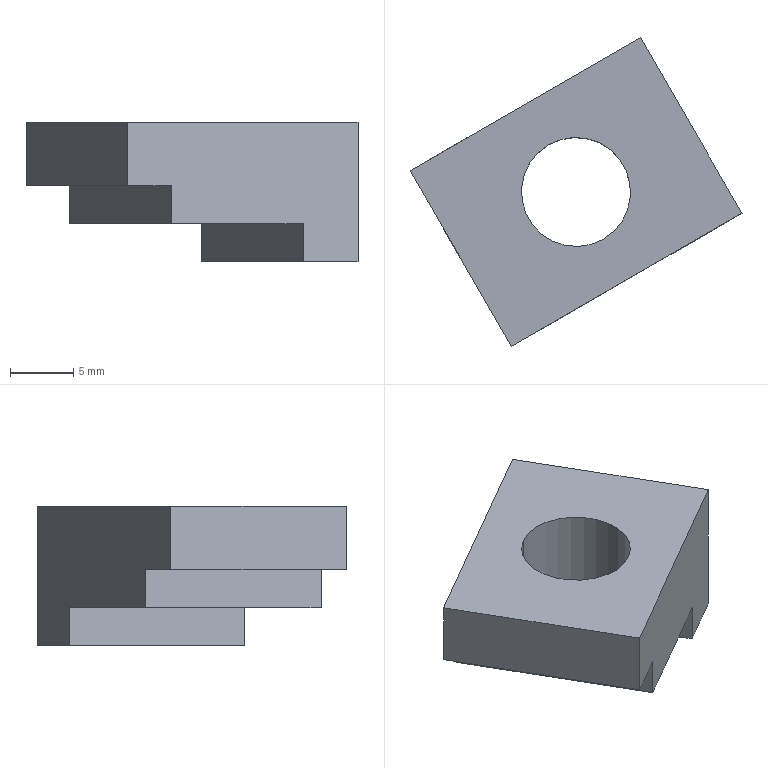Part | STEP file | 1_id1438_x_t | 1 solid | 12 faces | box 26.187 x 24.356 x 11 mm | volume 2271 mm3 | plane 10 | cylinder 2 | commonest cylinder face diameters 8.6 x2
STEP:
#1=CARTESIAN_POINT('',(0.,0.,0.));
#2=DIRECTION('',(0.,0.,1.));
#3=DIRECTION('',(1.,0.,0.));
#4=AXIS2_PLACEMENT_3D('',#1,#2,#3);
#5=CARTESIAN_POINT('',(88.803,28.678,51.075));
#6=VERTEX_POINT('',#5);
#7=CARTESIAN_POINT('',(96.803,14.822,51.075));
#8=VERTEX_POINT('',#7);
#9=CARTESIAN_POINT('',(88.803,28.678,51.075));
#10=DIRECTION('',(0.5,-0.866,0.));
#11=VECTOR('',#10,1.);
#12=LINE('',#9,#11);
#13=CARTESIAN_POINT('',(101.133,17.322,51.075));
#14=DIRECTION('',(0.,0.,1.));
#15=DIRECTION('',(-1.,0.,0.));
#16=AXIS2_PLACEMENT_3D('',#13,#14,#15);
#17=PLANE('',#16);
#18=CARTESIAN_POINT('',(12.33,-11.356));
#19=DIRECTION('',(-0.5,0.866));
#20=VECTOR('',#19,1.);
#21=LINE('',#18,#20);
#22=(GEOMETRIC_REPRESENTATION_CONTEXT(2)PARAMETRIC_REPRESENTATION_CONTEXT()REPRESENTATION_CONTEXT('',''));
#23=DEFINITIONAL_REPRESENTATION('',(#21),#22);
#24=PCURVE('',#17,#23);
#25=CARTESIAN_POINT('',(88.803,28.678,48.075));
#26=DIRECTION('',(-0.866,-0.5,0.));
#27=DIRECTION('',(0.5,-0.866,0.));
#28=AXIS2_PLACEMENT_3D('',#25,#26,#27);
#29=PLANE('',#28);
#30=CARTESIAN_POINT('',(0.,3.));
#31=DIRECTION('',(1.,0.));
#32=VECTOR('',#31,1.);
#33=LINE('',#30,#32);
#34=(GEOMETRIC_REPRESENTATION_CONTEXT(2)PARAMETRIC_REPRESENTATION_CONTEXT()REPRESENTATION_CONTEXT('',''));
#35=DEFINITIONAL_REPRESENTATION('',(#33),#34);
#36=PCURVE('',#29,#35);
#37=SURFACE_CURVE('',#12,(#24,#36),.PCURVE_S1.);
#38=EDGE_CURVE('',#6,#8,#37,.T.);
#39=ORIENTED_EDGE('',*,*,#38,.T.);
#40=CARTESIAN_POINT('',(86.411,8.822,51.075));
#41=VERTEX_POINT('',#40);
#42=CARTESIAN_POINT('',(96.803,14.822,51.075));
#43=DIRECTION('',(-0.866,-0.5,0.));
#44=VECTOR('',#43,1.);
#45=LINE('',#42,#44);
#46=CARTESIAN_POINT('',(4.33,2.5));
#47=DIRECTION('',(0.866,0.5));
#48=VECTOR('',#47,1.);
#49=LINE('',#46,#48);
#50=(GEOMETRIC_REPRESENTATION_CONTEXT(2)PARAMETRIC_REPRESENTATION_CONTEXT()REPRESENTATION_CONTEXT('',''));
#51=DEFINITIONAL_REPRESENTATION('',(#49),#50);
#52=PCURVE('',#17,#51);
#53=CARTESIAN_POINT('',(82.946,6.822,54.075));
#54=DIRECTION('',(0.5,-0.866,0.));
#55=DIRECTION('',(0.,0.,1.));
#56=AXIS2_PLACEMENT_3D('',#53,#54,#55);
#57=PLANE('',#56);
#58=CARTESIAN_POINT('',(-3.,-16.));
#59=DIRECTION('',(0.,1.));
#60=VECTOR('',#59,1.);
#61=LINE('',#58,#60);
#62=(GEOMETRIC_REPRESENTATION_CONTEXT(2)PARAMETRIC_REPRESENTATION_CONTEXT()REPRESENTATION_CONTEXT('',''));
#63=DEFINITIONAL_REPRESENTATION('',(#61),#62);
#64=PCURVE('',#57,#63);
#65=SURFACE_CURVE('',#45,(#52,#64),.PCURVE_S1.);
#66=EDGE_CURVE('',#8,#41,#65,.T.);
#67=ORIENTED_EDGE('',*,*,#66,.T.);
#68=CARTESIAN_POINT('',(78.411,22.678,51.075));
#69=VERTEX_POINT('',#68);
#70=CARTESIAN_POINT('',(86.411,8.822,51.075));
#71=DIRECTION('',(-0.5,0.866,0.));
#72=VECTOR('',#71,1.);
#73=LINE('',#70,#72);
#74=CARTESIAN_POINT('',(14.722,8.5));
#75=DIRECTION('',(0.5,-0.866));
#76=VECTOR('',#75,1.);
#77=LINE('',#74,#76);
#78=(GEOMETRIC_REPRESENTATION_CONTEXT(2)PARAMETRIC_REPRESENTATION_CONTEXT()REPRESENTATION_CONTEXT('',''));
#79=DEFINITIONAL_REPRESENTATION('',(#77),#78);
#80=PCURVE('',#17,#79);
#81=CARTESIAN_POINT('',(78.411,22.678,51.075));
#82=DIRECTION('',(-0.866,-0.5,0.));
#83=DIRECTION('',(0.5,-0.866,0.));
#84=AXIS2_PLACEMENT_3D('',#81,#82,#83);
#85=PLANE('',#84);
#86=CARTESIAN_POINT('',(16.,0.));
#87=DIRECTION('',(-1.,0.));
#88=VECTOR('',#87,1.);
#89=LINE('',#86,#88);
#90=(GEOMETRIC_REPRESENTATION_CONTEXT(2)PARAMETRIC_REPRESENTATION_CONTEXT()REPRESENTATION_CONTEXT('',''));
#91=DEFINITIONAL_REPRESENTATION('',(#89),#90);
#92=PCURVE('',#85,#91);
#93=SURFACE_CURVE('',#73,(#80,#92),.PCURVE_S1.);
#94=EDGE_CURVE('',#41,#69,#93,.T.);
#95=ORIENTED_EDGE('',*,*,#94,.T.);
#96=CARTESIAN_POINT('',(78.411,22.678,51.075));
#97=DIRECTION('',(0.866,0.5,0.));
#98=VECTOR('',#97,1.);
#99=LINE('',#96,#98);
#100=CARTESIAN_POINT('',(22.722,-5.356));
#101=DIRECTION('',(-0.866,-0.5));
#102=VECTOR('',#101,1.);
#103=LINE('',#100,#102);
#104=(GEOMETRIC_REPRESENTATION_CONTEXT(2)PARAMETRIC_REPRESENTATION_CONTEXT()REPRESENTATION_CONTEXT('',''));
#105=DEFINITIONAL_REPRESENTATION('',(#103),#104);
#106=PCURVE('',#17,#105);
#107=CARTESIAN_POINT('',(93.133,31.178,54.075));
#108=DIRECTION('',(-0.5,0.866,0.));
#109=DIRECTION('',(0.,0.,-1.));
#110=AXIS2_PLACEMENT_3D('',#107,#108,#109);
#111=PLANE('',#110);
#112=CARTESIAN_POINT('',(3.,17.));
#113=DIRECTION('',(0.,-1.));
#114=VECTOR('',#113,1.);
#115=LINE('',#112,#114);
#116=(GEOMETRIC_REPRESENTATION_CONTEXT(2)PARAMETRIC_REPRESENTATION_CONTEXT()REPRESENTATION_CONTEXT('',''));
#117=DEFINITIONAL_REPRESENTATION('',(#115),#116);
#118=PCURVE('',#111,#117);
#119=SURFACE_CURVE('',#99,(#106,#118),.PCURVE_S1.);
#120=EDGE_CURVE('',#69,#6,#119,.T.);
#121=ORIENTED_EDGE('',*,*,#120,.T.);
#122=EDGE_LOOP('',(#39,#67,#95,#121));
#123=FACE_BOUND('',#122,.T.);
#124=CARTESIAN_POINT('',(85.89,22.724,51.075));
#125=VERTEX_POINT('',#124);
#126=CARTESIAN_POINT('',(90.19,15.276,51.075));
#127=VERTEX_POINT('',#126);
#128=CARTESIAN_POINT('',(88.04,19.,51.075));
#129=DIRECTION('',(0.,0.,1.));
#130=DIRECTION('',(-0.5,0.866,0.));
#131=AXIS2_PLACEMENT_3D('',#128,#129,#130);
#132=CIRCLE('',#131,4.3);
#133=CARTESIAN_POINT('',(13.093,-1.678));
#134=DIRECTION('',(0.5,-0.866));
#135=AXIS2_PLACEMENT_2D('',#133,#134);
#136=CIRCLE('',#135,4.3);
#137=(GEOMETRIC_REPRESENTATION_CONTEXT(2)PARAMETRIC_REPRESENTATION_CONTEXT()REPRESENTATION_CONTEXT('',''));
#138=DEFINITIONAL_REPRESENTATION('',(#136),#137);
#139=PCURVE('',#17,#138);
#140=CARTESIAN_POINT('',(88.04,19.,31.155));
#141=DIRECTION('',(0.,0.,-1.));
#142=DIRECTION('',(0.5,-0.866,0.));
#143=AXIS2_PLACEMENT_3D('',#140,#141,#142);
#144=CYLINDRICAL_SURFACE('',#143,4.3);
#145=CARTESIAN_POINT('',(3.142,-19.92));
#146=DIRECTION('',(-1.,0.));
#147=VECTOR('',#146,1.);
#148=LINE('',#145,#147);
#149=(GEOMETRIC_REPRESENTATION_CONTEXT(2)PARAMETRIC_REPRESENTATION_CONTEXT()REPRESENTATION_CONTEXT('',''));
#150=DEFINITIONAL_REPRESENTATION('',(#148),#149);
#151=PCURVE('',#144,#150);
#152=SURFACE_CURVE('',#132,(#139,#151),.PCURVE_S1.);
#153=EDGE_CURVE('',#125,#127,#152,.T.);
#154=ORIENTED_EDGE('',*,*,#153,.T.);
#155=CARTESIAN_POINT('',(88.04,19.,51.075));
#156=DIRECTION('',(0.,0.,1.));
#157=DIRECTION('',(0.5,-0.866,0.));
#158=AXIS2_PLACEMENT_3D('',#155,#156,#157);
#159=CIRCLE('',#158,4.3);
#160=CARTESIAN_POINT('',(13.093,-1.678));
#161=DIRECTION('',(-0.5,0.866));
#162=AXIS2_PLACEMENT_2D('',#160,#161);
#163=CIRCLE('',#162,4.3);
#164=(GEOMETRIC_REPRESENTATION_CONTEXT(2)PARAMETRIC_REPRESENTATION_CONTEXT()REPRESENTATION_CONTEXT('',''));
#165=DEFINITIONAL_REPRESENTATION('',(#163),#164);
#166=PCURVE('',#17,#165);
#167=CARTESIAN_POINT('',(88.04,19.,31.155));
#168=DIRECTION('',(0.,0.,-1.));
#169=DIRECTION('',(0.5,-0.866,0.));
#170=AXIS2_PLACEMENT_3D('',#167,#168,#169);
#171=CYLINDRICAL_SURFACE('',#170,4.3);
#172=CARTESIAN_POINT('',(6.283,-19.92));
#173=DIRECTION('',(-1.,0.));
#174=VECTOR('',#173,1.);
#175=LINE('',#172,#174);
#176=(GEOMETRIC_REPRESENTATION_CONTEXT(2)PARAMETRIC_REPRESENTATION_CONTEXT()REPRESENTATION_CONTEXT('',''));
#177=DEFINITIONAL_REPRESENTATION('',(#175),#176);
#178=PCURVE('',#171,#177);
#179=SURFACE_CURVE('',#159,(#166,#178),.PCURVE_S1.);
#180=EDGE_CURVE('',#127,#125,#179,.T.);
#181=ORIENTED_EDGE('',*,*,#180,.T.);
#182=EDGE_LOOP('',(#154,#181));
#183=FACE_BOUND('',#182,.T.);
#184=ADVANCED_FACE('',(#123,#183),#17,.F.);
#185=CARTESIAN_POINT('',(93.133,31.178,59.075));
#186=VERTEX_POINT('',#185);
#187=CARTESIAN_POINT('',(74.946,20.678,59.075));
#188=VERTEX_POINT('',#187);
#189=CARTESIAN_POINT('',(93.133,31.178,59.075));
#190=DIRECTION('',(-0.866,-0.5,0.));
#191=VECTOR('',#190,1.);
#192=LINE('',#189,#191);
#193=CARTESIAN_POINT('',(-5.,0.));
#194=DIRECTION('',(0.,1.));
#195=VECTOR('',#194,1.);
#196=LINE('',#193,#195);
#197=(GEOMETRIC_REPRESENTATION_CONTEXT(2)PARAMETRIC_REPRESENTATION_CONTEXT()REPRESENTATION_CONTEXT('',''));
#198=DEFINITIONAL_REPRESENTATION('',(#196),#197);
#199=PCURVE('',#111,#198);
#200=CARTESIAN_POINT('',(74.946,20.678,59.075));
#201=DIRECTION('',(0.,0.,1.));
#202=DIRECTION('',(-1.,0.,0.));
#203=AXIS2_PLACEMENT_3D('',#200,#201,#202);
#204=PLANE('',#203);
#205=CARTESIAN_POINT('',(-18.187,-10.5));
#206=DIRECTION('',(0.866,0.5));
#207=VECTOR('',#206,1.);
#208=LINE('',#205,#207);
#209=(GEOMETRIC_REPRESENTATION_CONTEXT(2)PARAMETRIC_REPRESENTATION_CONTEXT()REPRESENTATION_CONTEXT('',''));
#210=DEFINITIONAL_REPRESENTATION('',(#208),#209);
#211=PCURVE('',#204,#210);
#212=SURFACE_CURVE('',#192,(#199,#211),.PCURVE_S1.);
#213=EDGE_CURVE('',#186,#188,#212,.T.);
#214=ORIENTED_EDGE('',*,*,#213,.F.);
#215=CARTESIAN_POINT('',(93.133,31.178,48.075));
#216=VERTEX_POINT('',#215);
#217=CARTESIAN_POINT('',(93.133,31.178,59.075));
#218=DIRECTION('',(0.,0.,-1.));
#219=VECTOR('',#218,1.);
#220=LINE('',#217,#219);
#221=CARTESIAN_POINT('',(-5.,0.));
#222=DIRECTION('',(1.,0.));
#223=VECTOR('',#222,1.);
#224=LINE('',#221,#223);
#225=(GEOMETRIC_REPRESENTATION_CONTEXT(2)PARAMETRIC_REPRESENTATION_CONTEXT()REPRESENTATION_CONTEXT('',''));
#226=DEFINITIONAL_REPRESENTATION('',(#224),#225);
#227=PCURVE('',#111,#226);
#228=CARTESIAN_POINT('',(101.133,17.322,54.075));
#229=DIRECTION('',(0.866,0.5,0.));
#230=DIRECTION('',(0.,0.,1.));
#231=AXIS2_PLACEMENT_3D('',#228,#229,#230);
#232=PLANE('',#231);
#233=CARTESIAN_POINT('',(5.,-16.));
#234=DIRECTION('',(-1.,0.));
#235=VECTOR('',#234,1.);
#236=LINE('',#233,#235);
#237=(GEOMETRIC_REPRESENTATION_CONTEXT(2)PARAMETRIC_REPRESENTATION_CONTEXT()REPRESENTATION_CONTEXT('',''));
#238=DEFINITIONAL_REPRESENTATION('',(#236),#237);
#239=PCURVE('',#232,#238);
#240=SURFACE_CURVE('',#220,(#227,#239),.PCURVE_S1.);
#241=EDGE_CURVE('',#186,#216,#240,.T.);
#242=ORIENTED_EDGE('',*,*,#241,.T.);
#243=CARTESIAN_POINT('',(88.803,28.678,48.075));
#244=VERTEX_POINT('',#243);
#245=CARTESIAN_POINT('',(88.803,28.678,48.075));
#246=DIRECTION('',(0.866,0.5,0.));
#247=VECTOR('',#246,1.);
#248=LINE('',#245,#247);
#249=CARTESIAN_POINT('',(6.,5.));
#250=DIRECTION('',(0.,-1.));
#251=VECTOR('',#250,1.);
#252=LINE('',#249,#251);
#253=(GEOMETRIC_REPRESENTATION_CONTEXT(2)PARAMETRIC_REPRESENTATION_CONTEXT()REPRESENTATION_CONTEXT('',''));
#254=DEFINITIONAL_REPRESENTATION('',(#252),#253);
#255=PCURVE('',#111,#254);
#256=CARTESIAN_POINT('',(101.133,17.322,48.075));
#257=DIRECTION('',(0.,0.,1.));
#258=DIRECTION('',(-1.,0.,0.));
#259=AXIS2_PLACEMENT_3D('',#256,#257,#258);
#260=PLANE('',#259);
#261=CARTESIAN_POINT('',(12.33,-11.356));
#262=DIRECTION('',(-0.866,-0.5));
#263=VECTOR('',#262,1.);
#264=LINE('',#261,#263);
#265=(GEOMETRIC_REPRESENTATION_CONTEXT(2)PARAMETRIC_REPRESENTATION_CONTEXT()REPRESENTATION_CONTEXT('',''));
#266=DEFINITIONAL_REPRESENTATION('',(#264),#265);
#267=PCURVE('',#260,#266);
#268=SURFACE_CURVE('',#248,(#255,#267),.PCURVE_S1.);
#269=EDGE_CURVE('',#244,#216,#268,.T.);
#270=ORIENTED_EDGE('',*,*,#269,.F.);
#271=CARTESIAN_POINT('',(88.803,28.678,51.075));
#272=DIRECTION('',(0.,0.,-1.));
#273=VECTOR('',#272,1.);
#274=LINE('',#271,#273);
#275=CARTESIAN_POINT('',(3.,5.));
#276=DIRECTION('',(1.,0.));
#277=VECTOR('',#276,1.);
#278=LINE('',#275,#277);
#279=(GEOMETRIC_REPRESENTATION_CONTEXT(2)PARAMETRIC_REPRESENTATION_CONTEXT()REPRESENTATION_CONTEXT('',''));
#280=DEFINITIONAL_REPRESENTATION('',(#278),#279);
#281=PCURVE('',#111,#280);
#282=CARTESIAN_POINT('',(0.,3.));
#283=DIRECTION('',(0.,-1.));
#284=VECTOR('',#283,1.);
#285=LINE('',#282,#284);
#286=(GEOMETRIC_REPRESENTATION_CONTEXT(2)PARAMETRIC_REPRESENTATION_CONTEXT()REPRESENTATION_CONTEXT('',''));
#287=DEFINITIONAL_REPRESENTATION('',(#285),#286);
#288=PCURVE('',#29,#287);
#289=SURFACE_CURVE('',#274,(#281,#288),.PCURVE_S1.);
#290=EDGE_CURVE('',#6,#244,#289,.T.);
#291=ORIENTED_EDGE('',*,*,#290,.F.);
#292=ORIENTED_EDGE('',*,*,#120,.F.);
#293=CARTESIAN_POINT('',(78.411,22.678,54.075));
#294=VERTEX_POINT('',#293);
#295=CARTESIAN_POINT('',(78.411,22.678,54.075));
#296=DIRECTION('',(0.,0.,-1.));
#297=VECTOR('',#296,1.);
#298=LINE('',#295,#297);
#299=CARTESIAN_POINT('',(0.,17.));
#300=DIRECTION('',(1.,0.));
#301=VECTOR('',#300,1.);
#302=LINE('',#299,#301);
#303=(GEOMETRIC_REPRESENTATION_CONTEXT(2)PARAMETRIC_REPRESENTATION_CONTEXT()REPRESENTATION_CONTEXT('',''));
#304=DEFINITIONAL_REPRESENTATION('',(#302),#303);
#305=PCURVE('',#111,#304);
#306=CARTESIAN_POINT('',(0.,3.));
#307=DIRECTION('',(0.,-1.));
#308=VECTOR('',#307,1.);
#309=LINE('',#306,#308);
#310=(GEOMETRIC_REPRESENTATION_CONTEXT(2)PARAMETRIC_REPRESENTATION_CONTEXT()REPRESENTATION_CONTEXT('',''));
#311=DEFINITIONAL_REPRESENTATION('',(#309),#310);
#312=PCURVE('',#85,#311);
#313=SURFACE_CURVE('',#298,(#305,#312),.PCURVE_S1.);
#314=EDGE_CURVE('',#294,#69,#313,.T.);
#315=ORIENTED_EDGE('',*,*,#314,.F.);
#316=CARTESIAN_POINT('',(74.946,20.678,54.075));
#317=VERTEX_POINT('',#316);
#318=CARTESIAN_POINT('',(74.946,20.678,54.075));
#319=DIRECTION('',(0.866,0.5,0.));
#320=VECTOR('',#319,1.);
#321=LINE('',#318,#320);
#322=CARTESIAN_POINT('',(0.,21.));
#323=DIRECTION('',(0.,-1.));
#324=VECTOR('',#323,1.);
#325=LINE('',#322,#324);
#326=(GEOMETRIC_REPRESENTATION_CONTEXT(2)PARAMETRIC_REPRESENTATION_CONTEXT()REPRESENTATION_CONTEXT('',''));
#327=DEFINITIONAL_REPRESENTATION('',(#325),#326);
#328=PCURVE('',#111,#327);
#329=CARTESIAN_POINT('',(74.946,20.678,54.075));
#330=DIRECTION('',(0.,0.,1.));
#331=DIRECTION('',(-1.,0.,0.));
#332=AXIS2_PLACEMENT_3D('',#329,#330,#331);
#333=PLANE('',#332);
#334=CARTESIAN_POINT('',(0.,0.));
#335=DIRECTION('',(-0.866,-0.5));
#336=VECTOR('',#335,1.);
#337=LINE('',#334,#336);
#338=(GEOMETRIC_REPRESENTATION_CONTEXT(2)PARAMETRIC_REPRESENTATION_CONTEXT()REPRESENTATION_CONTEXT('',''));
#339=DEFINITIONAL_REPRESENTATION('',(#337),#338);
#340=PCURVE('',#333,#339);
#341=SURFACE_CURVE('',#321,(#328,#340),.PCURVE_S1.);
#342=EDGE_CURVE('',#317,#294,#341,.T.);
#343=ORIENTED_EDGE('',*,*,#342,.F.);
#344=CARTESIAN_POINT('',(74.946,20.678,59.075));
#345=DIRECTION('',(0.,0.,-1.));
#346=VECTOR('',#345,1.);
#347=LINE('',#344,#346);
#348=CARTESIAN_POINT('',(-5.,21.));
#349=DIRECTION('',(1.,0.));
#350=VECTOR('',#349,1.);
#351=LINE('',#348,#350);
#352=(GEOMETRIC_REPRESENTATION_CONTEXT(2)PARAMETRIC_REPRESENTATION_CONTEXT()REPRESENTATION_CONTEXT('',''));
#353=DEFINITIONAL_REPRESENTATION('',(#351),#352);
#354=PCURVE('',#111,#353);
#355=CARTESIAN_POINT('',(74.946,20.678,54.075));
#356=DIRECTION('',(-0.866,-0.5,0.));
#357=DIRECTION('',(0.5,-0.866,0.));
#358=AXIS2_PLACEMENT_3D('',#355,#356,#357);
#359=PLANE('',#358);
#360=CARTESIAN_POINT('',(0.,5.));
#361=DIRECTION('',(0.,-1.));
#362=VECTOR('',#361,1.);
#363=LINE('',#360,#362);
#364=(GEOMETRIC_REPRESENTATION_CONTEXT(2)PARAMETRIC_REPRESENTATION_CONTEXT()REPRESENTATION_CONTEXT('',''));
#365=DEFINITIONAL_REPRESENTATION('',(#363),#364);
#366=PCURVE('',#359,#365);
#367=SURFACE_CURVE('',#347,(#354,#366),.PCURVE_S1.);
#368=EDGE_CURVE('',#188,#317,#367,.T.);
#369=ORIENTED_EDGE('',*,*,#368,.F.);
#370=EDGE_LOOP('',(#214,#242,#270,#291,#292,#315,#343,#369));
#371=FACE_BOUND('',#370,.T.);
#372=ADVANCED_FACE('',(#371),#111,.T.);
#373=ORIENTED_EDGE('',*,*,#368,.T.);
#374=CARTESIAN_POINT('',(82.946,6.822,54.075));
#375=VERTEX_POINT('',#374);
#376=CARTESIAN_POINT('',(82.946,6.822,54.075));
#377=DIRECTION('',(-0.5,0.866,0.));
#378=VECTOR('',#377,1.);
#379=LINE('',#376,#378);
#380=CARTESIAN_POINT('',(16.,0.));
#381=DIRECTION('',(-1.,0.));
#382=VECTOR('',#381,1.);
#383=LINE('',#380,#382);
#384=(GEOMETRIC_REPRESENTATION_CONTEXT(2)PARAMETRIC_REPRESENTATION_CONTEXT()REPRESENTATION_CONTEXT('',''));
#385=DEFINITIONAL_REPRESENTATION('',(#383),#384);
#386=PCURVE('',#359,#385);
#387=CARTESIAN_POINT('',(-8.,13.856));
#388=DIRECTION('',(0.5,-0.866));
#389=VECTOR('',#388,1.);
#390=LINE('',#387,#389);
#391=(GEOMETRIC_REPRESENTATION_CONTEXT(2)PARAMETRIC_REPRESENTATION_CONTEXT()REPRESENTATION_CONTEXT('',''));
#392=DEFINITIONAL_REPRESENTATION('',(#390),#391);
#393=PCURVE('',#333,#392);
#394=SURFACE_CURVE('',#379,(#386,#393),.PCURVE_S1.);
#395=EDGE_CURVE('',#375,#317,#394,.T.);
#396=ORIENTED_EDGE('',*,*,#395,.F.);
#397=CARTESIAN_POINT('',(82.946,6.822,59.075));
#398=VERTEX_POINT('',#397);
#399=CARTESIAN_POINT('',(82.946,6.822,59.075));
#400=DIRECTION('',(0.,0.,-1.));
#401=VECTOR('',#400,1.);
#402=LINE('',#399,#401);
#403=CARTESIAN_POINT('',(16.,5.));
#404=DIRECTION('',(0.,-1.));
#405=VECTOR('',#404,1.);
#406=LINE('',#403,#405);
#407=(GEOMETRIC_REPRESENTATION_CONTEXT(2)PARAMETRIC_REPRESENTATION_CONTEXT()REPRESENTATION_CONTEXT('',''));
#408=DEFINITIONAL_REPRESENTATION('',(#406),#407);
#409=PCURVE('',#359,#408);
#410=CARTESIAN_POINT('',(5.,0.));
#411=DIRECTION('',(-1.,0.));
#412=VECTOR('',#411,1.);
#413=LINE('',#410,#412);
#414=(GEOMETRIC_REPRESENTATION_CONTEXT(2)PARAMETRIC_REPRESENTATION_CONTEXT()REPRESENTATION_CONTEXT('',''));
#415=DEFINITIONAL_REPRESENTATION('',(#413),#414);
#416=PCURVE('',#57,#415);
#417=SURFACE_CURVE('',#402,(#409,#416),.PCURVE_S1.);
#418=EDGE_CURVE('',#398,#375,#417,.T.);
#419=ORIENTED_EDGE('',*,*,#418,.F.);
#420=CARTESIAN_POINT('',(74.946,20.678,59.075));
#421=DIRECTION('',(0.5,-0.866,0.));
#422=VECTOR('',#421,1.);
#423=LINE('',#420,#422);
#424=CARTESIAN_POINT('',(0.,5.));
#425=DIRECTION('',(1.,0.));
#426=VECTOR('',#425,1.);
#427=LINE('',#424,#426);
#428=(GEOMETRIC_REPRESENTATION_CONTEXT(2)PARAMETRIC_REPRESENTATION_CONTEXT()REPRESENTATION_CONTEXT('',''));
#429=DEFINITIONAL_REPRESENTATION('',(#427),#428);
#430=PCURVE('',#359,#429);
#431=CARTESIAN_POINT('',(0.,0.));
#432=DIRECTION('',(-0.5,0.866));
#433=VECTOR('',#432,1.);
#434=LINE('',#431,#433);
#435=(GEOMETRIC_REPRESENTATION_CONTEXT(2)PARAMETRIC_REPRESENTATION_CONTEXT()REPRESENTATION_CONTEXT('',''));
#436=DEFINITIONAL_REPRESENTATION('',(#434),#435);
#437=PCURVE('',#204,#436);
#438=SURFACE_CURVE('',#423,(#430,#437),.PCURVE_S1.);
#439=EDGE_CURVE('',#188,#398,#438,.T.);
#440=ORIENTED_EDGE('',*,*,#439,.F.);
#441=EDGE_LOOP('',(#373,#396,#419,#440));
#442=FACE_BOUND('',#441,.T.);
#443=ADVANCED_FACE('',(#442),#359,.T.);
#444=CARTESIAN_POINT('',(101.133,17.322,59.075));
#445=VERTEX_POINT('',#444);
#446=CARTESIAN_POINT('',(101.133,17.322,59.075));
#447=DIRECTION('',(-0.5,0.866,0.));
#448=VECTOR('',#447,1.);
#449=LINE('',#446,#448);
#450=CARTESIAN_POINT('',(-26.187,3.356));
#451=DIRECTION('',(0.5,-0.866));
#452=VECTOR('',#451,1.);
#453=LINE('',#450,#452);
#454=(GEOMETRIC_REPRESENTATION_CONTEXT(2)PARAMETRIC_REPRESENTATION_CONTEXT()REPRESENTATION_CONTEXT('',''));
#455=DEFINITIONAL_REPRESENTATION('',(#453),#454);
#456=PCURVE('',#204,#455);
#457=CARTESIAN_POINT('',(5.,0.));
#458=DIRECTION('',(0.,-1.));
#459=VECTOR('',#458,1.);
#460=LINE('',#457,#459);
#461=(GEOMETRIC_REPRESENTATION_CONTEXT(2)PARAMETRIC_REPRESENTATION_CONTEXT()REPRESENTATION_CONTEXT('',''));
#462=DEFINITIONAL_REPRESENTATION('',(#460),#461);
#463=PCURVE('',#232,#462);
#464=SURFACE_CURVE('',#449,(#456,#463),.PCURVE_S1.);
#465=EDGE_CURVE('',#445,#186,#464,.T.);
#466=ORIENTED_EDGE('',*,*,#465,.T.);
#467=ORIENTED_EDGE('',*,*,#213,.T.);
#468=ORIENTED_EDGE('',*,*,#439,.T.);
#469=CARTESIAN_POINT('',(82.946,6.822,59.075));
#470=DIRECTION('',(0.866,0.5,0.));
#471=VECTOR('',#470,1.);
#472=LINE('',#469,#471);
#473=CARTESIAN_POINT('',(-8.,13.856));
#474=DIRECTION('',(-0.866,-0.5));
#475=VECTOR('',#474,1.);
#476=LINE('',#473,#475);
#477=(GEOMETRIC_REPRESENTATION_CONTEXT(2)PARAMETRIC_REPRESENTATION_CONTEXT()REPRESENTATION_CONTEXT('',''));
#478=DEFINITIONAL_REPRESENTATION('',(#476),#477);
#479=PCURVE('',#204,#478);
#480=CARTESIAN_POINT('',(5.,0.));
#481=DIRECTION('',(0.,-1.));
#482=VECTOR('',#481,1.);
#483=LINE('',#480,#482);
#484=(GEOMETRIC_REPRESENTATION_CONTEXT(2)PARAMETRIC_REPRESENTATION_CONTEXT()REPRESENTATION_CONTEXT('',''));
#485=DEFINITIONAL_REPRESENTATION('',(#483),#484);
#486=PCURVE('',#57,#485);
#487=SURFACE_CURVE('',#472,(#479,#486),.PCURVE_S1.);
#488=EDGE_CURVE('',#398,#445,#487,.T.);
#489=ORIENTED_EDGE('',*,*,#488,.T.);
#490=EDGE_LOOP('',(#466,#467,#468,#489));
#491=FACE_BOUND('',#490,.T.);
#492=CARTESIAN_POINT('',(85.89,22.724,59.075));
#493=VERTEX_POINT('',#492);
#494=CARTESIAN_POINT('',(90.19,15.276,59.075));
#495=VERTEX_POINT('',#494);
#496=CARTESIAN_POINT('',(88.04,19.,59.075));
#497=DIRECTION('',(0.,0.,-1.));
#498=DIRECTION('',(-0.5,0.866,0.));
#499=AXIS2_PLACEMENT_3D('',#496,#497,#498);
#500=CIRCLE('',#499,4.3);
#501=CARTESIAN_POINT('',(-10.943,-2.046));
#502=CARTESIAN_POINT('',(-17.393,-5.77));
#503=CARTESIAN_POINT('',(-17.393,1.678));
#504=CARTESIAN_POINT('',(-17.393,9.126));
#505=CARTESIAN_POINT('',(-10.943,5.402));
#506=CARTESIAN_POINT('',(-4.493,1.678));
#507=CARTESIAN_POINT('',(-10.943,-2.046));
#508=(BOUNDED_CURVE()B_SPLINE_CURVE(2,(#501,#502,#503,#504,#505,#506,#507),.UNSPECIFIED.,.T.,.F.)B_SPLINE_CURVE_WITH_KNOTS((1,2,2,2,2,1),(-2.094,0.,2.094,4.189,6.283,8.378),.UNSPECIFIED.)CURVE()GEOMETRIC_REPRESENTATION_ITEM()RATIONAL_B_SPLINE_CURVE((1.,0.5,1.,0.5,1.,0.5,1.))REPRESENTATION_ITEM(''));
#509=(GEOMETRIC_REPRESENTATION_CONTEXT(2)PARAMETRIC_REPRESENTATION_CONTEXT()REPRESENTATION_CONTEXT('',''));
#510=DEFINITIONAL_REPRESENTATION('',(#508),#509);
#511=PCURVE('',#204,#510);
#512=CARTESIAN_POINT('',(3.142,-27.92));
#513=DIRECTION('',(1.,0.));
#514=VECTOR('',#513,1.);
#515=LINE('',#512,#514);
#516=(GEOMETRIC_REPRESENTATION_CONTEXT(2)PARAMETRIC_REPRESENTATION_CONTEXT()REPRESENTATION_CONTEXT('',''));
#517=DEFINITIONAL_REPRESENTATION('',(#515),#516);
#518=PCURVE('',#171,#517);
#519=SURFACE_CURVE('',#500,(#511,#518),.PCURVE_S1.);
#520=EDGE_CURVE('',#493,#495,#519,.T.);
#521=ORIENTED_EDGE('',*,*,#520,.T.);
#522=CARTESIAN_POINT('',(88.04,19.,59.075));
#523=DIRECTION('',(0.,0.,-1.));
#524=DIRECTION('',(0.5,-0.866,0.));
#525=AXIS2_PLACEMENT_3D('',#522,#523,#524);
#526=CIRCLE('',#525,4.3);
#527=CARTESIAN_POINT('',(-15.243,5.402));
#528=CARTESIAN_POINT('',(-8.793,9.126));
#529=CARTESIAN_POINT('',(-8.793,1.678));
#530=CARTESIAN_POINT('',(-8.793,-5.77));
#531=CARTESIAN_POINT('',(-15.243,-2.046));
#532=CARTESIAN_POINT('',(-21.693,1.678));
#533=CARTESIAN_POINT('',(-15.243,5.402));
#534=(BOUNDED_CURVE()B_SPLINE_CURVE(2,(#527,#528,#529,#530,#531,#532,#533),.UNSPECIFIED.,.T.,.F.)B_SPLINE_CURVE_WITH_KNOTS((1,2,2,2,2,1),(-2.094,0.,2.094,4.189,6.283,8.378),.UNSPECIFIED.)CURVE()GEOMETRIC_REPRESENTATION_ITEM()RATIONAL_B_SPLINE_CURVE((1.,0.5,1.,0.5,1.,0.5,1.))REPRESENTATION_ITEM(''));
#535=(GEOMETRIC_REPRESENTATION_CONTEXT(2)PARAMETRIC_REPRESENTATION_CONTEXT()REPRESENTATION_CONTEXT('',''));
#536=DEFINITIONAL_REPRESENTATION('',(#534),#535);
#537=PCURVE('',#204,#536);
#538=CARTESIAN_POINT('',(0.,-27.92));
#539=DIRECTION('',(1.,0.));
#540=VECTOR('',#539,1.);
#541=LINE('',#538,#540);
#542=(GEOMETRIC_REPRESENTATION_CONTEXT(2)PARAMETRIC_REPRESENTATION_CONTEXT()REPRESENTATION_CONTEXT('',''));
#543=DEFINITIONAL_REPRESENTATION('',(#541),#542);
#544=PCURVE('',#144,#543);
#545=SURFACE_CURVE('',#526,(#537,#544),.PCURVE_S1.);
#546=EDGE_CURVE('',#495,#493,#545,.T.);
#547=ORIENTED_EDGE('',*,*,#546,.T.);
#548=EDGE_LOOP('',(#521,#547));
#549=FACE_BOUND('',#548,.T.);
#550=ADVANCED_FACE('',(#491,#549),#204,.T.);
#551=CARTESIAN_POINT('',(96.803,14.822,48.075));
#552=VERTEX_POINT('',#551);
#553=CARTESIAN_POINT('',(96.803,14.822,51.075));
#554=DIRECTION('',(0.,0.,-1.));
#555=VECTOR('',#554,1.);
#556=LINE('',#553,#555);
#557=CARTESIAN_POINT('',(-3.,-16.));
#558=DIRECTION('',(-1.,0.));
#559=VECTOR('',#558,1.);
#560=LINE('',#557,#559);
#561=(GEOMETRIC_REPRESENTATION_CONTEXT(2)PARAMETRIC_REPRESENTATION_CONTEXT()REPRESENTATION_CONTEXT('',''));
#562=DEFINITIONAL_REPRESENTATION('',(#560),#561);
#563=PCURVE('',#57,#562);
#564=CARTESIAN_POINT('',(16.,3.));
#565=DIRECTION('',(0.,-1.));
#566=VECTOR('',#565,1.);
#567=LINE('',#564,#566);
#568=(GEOMETRIC_REPRESENTATION_CONTEXT(2)PARAMETRIC_REPRESENTATION_CONTEXT()REPRESENTATION_CONTEXT('',''));
#569=DEFINITIONAL_REPRESENTATION('',(#567),#568);
#570=PCURVE('',#29,#569);
#571=SURFACE_CURVE('',#556,(#563,#570),.PCURVE_S1.);
#572=EDGE_CURVE('',#8,#552,#571,.T.);
#573=ORIENTED_EDGE('',*,*,#572,.T.);
#574=CARTESIAN_POINT('',(101.133,17.322,48.075));
#575=VERTEX_POINT('',#574);
#576=CARTESIAN_POINT('',(101.133,17.322,48.075));
#577=DIRECTION('',(-0.866,-0.5,0.));
#578=VECTOR('',#577,1.);
#579=LINE('',#576,#578);
#580=CARTESIAN_POINT('',(-6.,-21.));
#581=DIRECTION('',(0.,1.));
#582=VECTOR('',#581,1.);
#583=LINE('',#580,#582);
#584=(GEOMETRIC_REPRESENTATION_CONTEXT(2)PARAMETRIC_REPRESENTATION_CONTEXT()REPRESENTATION_CONTEXT('',''));
#585=DEFINITIONAL_REPRESENTATION('',(#583),#584);
#586=PCURVE('',#57,#585);
#587=CARTESIAN_POINT('',(0.,0.));
#588=DIRECTION('',(0.866,0.5));
#589=VECTOR('',#588,1.);
#590=LINE('',#587,#589);
#591=(GEOMETRIC_REPRESENTATION_CONTEXT(2)PARAMETRIC_REPRESENTATION_CONTEXT()REPRESENTATION_CONTEXT('',''));
#592=DEFINITIONAL_REPRESENTATION('',(#590),#591);
#593=PCURVE('',#260,#592);
#594=SURFACE_CURVE('',#579,(#586,#593),.PCURVE_S1.);
#595=EDGE_CURVE('',#575,#552,#594,.T.);
#596=ORIENTED_EDGE('',*,*,#595,.F.);
#597=CARTESIAN_POINT('',(101.133,17.322,59.075));
#598=DIRECTION('',(0.,0.,-1.));
#599=VECTOR('',#598,1.);
#600=LINE('',#597,#599);
#601=CARTESIAN_POINT('',(5.,-21.));
#602=DIRECTION('',(-1.,0.));
#603=VECTOR('',#602,1.);
#604=LINE('',#601,#603);
#605=(GEOMETRIC_REPRESENTATION_CONTEXT(2)PARAMETRIC_REPRESENTATION_CONTEXT()REPRESENTATION_CONTEXT('',''));
#606=DEFINITIONAL_REPRESENTATION('',(#604),#605);
#607=PCURVE('',#57,#606);
#608=CARTESIAN_POINT('',(5.,0.));
#609=DIRECTION('',(-1.,0.));
#610=VECTOR('',#609,1.);
#611=LINE('',#608,#610);
#612=(GEOMETRIC_REPRESENTATION_CONTEXT(2)PARAMETRIC_REPRESENTATION_CONTEXT()REPRESENTATION_CONTEXT('',''));
#613=DEFINITIONAL_REPRESENTATION('',(#611),#612);
#614=PCURVE('',#232,#613);
#615=SURFACE_CURVE('',#600,(#607,#614),.PCURVE_S1.);
#616=EDGE_CURVE('',#445,#575,#615,.T.);
#617=ORIENTED_EDGE('',*,*,#616,.F.);
#618=ORIENTED_EDGE('',*,*,#488,.F.);
#619=ORIENTED_EDGE('',*,*,#418,.T.);
#620=CARTESIAN_POINT('',(86.411,8.822,54.075));
#621=VERTEX_POINT('',#620);
#622=CARTESIAN_POINT('',(86.411,8.822,54.075));
#623=DIRECTION('',(-0.866,-0.5,0.));
#624=VECTOR('',#623,1.);
#625=LINE('',#622,#624);
#626=CARTESIAN_POINT('',(0.,-4.));
#627=DIRECTION('',(0.,1.));
#628=VECTOR('',#627,1.);
#629=LINE('',#626,#628);
#630=(GEOMETRIC_REPRESENTATION_CONTEXT(2)PARAMETRIC_REPRESENTATION_CONTEXT()REPRESENTATION_CONTEXT('',''));
#631=DEFINITIONAL_REPRESENTATION('',(#629),#630);
#632=PCURVE('',#57,#631);
#633=CARTESIAN_POINT('',(-11.464,11.856));
#634=DIRECTION('',(0.866,0.5));
#635=VECTOR('',#634,1.);
#636=LINE('',#633,#635);
#637=(GEOMETRIC_REPRESENTATION_CONTEXT(2)PARAMETRIC_REPRESENTATION_CONTEXT()REPRESENTATION_CONTEXT('',''));
#638=DEFINITIONAL_REPRESENTATION('',(#636),#637);
#639=PCURVE('',#333,#638);
#640=SURFACE_CURVE('',#625,(#632,#639),.PCURVE_S1.);
#641=EDGE_CURVE('',#621,#375,#640,.T.);
#642=ORIENTED_EDGE('',*,*,#641,.F.);
#643=CARTESIAN_POINT('',(86.411,8.822,54.075));
#644=DIRECTION('',(0.,0.,-1.));
#645=VECTOR('',#644,1.);
#646=LINE('',#643,#645);
#647=CARTESIAN_POINT('',(0.,-4.));
#648=DIRECTION('',(-1.,0.));
#649=VECTOR('',#648,1.);
#650=LINE('',#647,#649);
#651=(GEOMETRIC_REPRESENTATION_CONTEXT(2)PARAMETRIC_REPRESENTATION_CONTEXT()REPRESENTATION_CONTEXT('',''));
#652=DEFINITIONAL_REPRESENTATION('',(#650),#651);
#653=PCURVE('',#57,#652);
#654=CARTESIAN_POINT('',(16.,3.));
#655=DIRECTION('',(0.,-1.));
#656=VECTOR('',#655,1.);
#657=LINE('',#654,#656);
#658=(GEOMETRIC_REPRESENTATION_CONTEXT(2)PARAMETRIC_REPRESENTATION_CONTEXT()REPRESENTATION_CONTEXT('',''));
#659=DEFINITIONAL_REPRESENTATION('',(#657),#658);
#660=PCURVE('',#85,#659);
#661=SURFACE_CURVE('',#646,(#653,#660),.PCURVE_S1.);
#662=EDGE_CURVE('',#621,#41,#661,.T.);
#663=ORIENTED_EDGE('',*,*,#662,.T.);
#664=ORIENTED_EDGE('',*,*,#66,.F.);
#665=EDGE_LOOP('',(#573,#596,#617,#618,#619,#642,#663,#664));
#666=FACE_BOUND('',#665,.T.);
#667=ADVANCED_FACE('',(#666),#57,.T.);
#668=ORIENTED_EDGE('',*,*,#314,.T.);
#669=ORIENTED_EDGE('',*,*,#94,.F.);
#670=ORIENTED_EDGE('',*,*,#662,.F.);
#671=CARTESIAN_POINT('',(78.411,22.678,54.075));
#672=DIRECTION('',(0.5,-0.866,0.));
#673=VECTOR('',#672,1.);
#674=LINE('',#671,#673);
#675=CARTESIAN_POINT('',(0.,3.));
#676=DIRECTION('',(1.,0.));
#677=VECTOR('',#676,1.);
#678=LINE('',#675,#677);
#679=(GEOMETRIC_REPRESENTATION_CONTEXT(2)PARAMETRIC_REPRESENTATION_CONTEXT()REPRESENTATION_CONTEXT('',''));
#680=DEFINITIONAL_REPRESENTATION('',(#678),#679);
#681=PCURVE('',#85,#680);
#682=CARTESIAN_POINT('',(-3.464,-2.));
#683=DIRECTION('',(-0.5,0.866));
#684=VECTOR('',#683,1.);
#685=LINE('',#682,#684);
#686=(GEOMETRIC_REPRESENTATION_CONTEXT(2)PARAMETRIC_REPRESENTATION_CONTEXT()REPRESENTATION_CONTEXT('',''));
#687=DEFINITIONAL_REPRESENTATION('',(#685),#686);
#688=PCURVE('',#333,#687);
#689=SURFACE_CURVE('',#674,(#681,#688),.PCURVE_S1.);
#690=EDGE_CURVE('',#294,#621,#689,.T.);
#691=ORIENTED_EDGE('',*,*,#690,.F.);
#692=EDGE_LOOP('',(#668,#669,#670,#691));
#693=FACE_BOUND('',#692,.T.);
#694=ADVANCED_FACE('',(#693),#85,.T.);
#695=ORIENTED_EDGE('',*,*,#690,.T.);
#696=ORIENTED_EDGE('',*,*,#641,.T.);
#697=ORIENTED_EDGE('',*,*,#395,.T.);
#698=ORIENTED_EDGE('',*,*,#342,.T.);
#699=EDGE_LOOP('',(#695,#696,#697,#698));
#700=FACE_BOUND('',#699,.T.);
#701=ADVANCED_FACE('',(#700),#333,.F.);
#702=ORIENTED_EDGE('',*,*,#616,.T.);
#703=CARTESIAN_POINT('',(93.133,31.178,48.075));
#704=DIRECTION('',(0.5,-0.866,0.));
#705=VECTOR('',#704,1.);
#706=LINE('',#703,#705);
#707=CARTESIAN_POINT('',(-6.,-16.));
#708=DIRECTION('',(0.,1.));
#709=VECTOR('',#708,1.);
#710=LINE('',#707,#709);
#711=(GEOMETRIC_REPRESENTATION_CONTEXT(2)PARAMETRIC_REPRESENTATION_CONTEXT()REPRESENTATION_CONTEXT('',''));
#712=DEFINITIONAL_REPRESENTATION('',(#710),#711);
#713=PCURVE('',#232,#712);
#714=CARTESIAN_POINT('',(8.,-13.856));
#715=DIRECTION('',(-0.5,0.866));
#716=VECTOR('',#715,1.);
#717=LINE('',#714,#716);
#718=(GEOMETRIC_REPRESENTATION_CONTEXT(2)PARAMETRIC_REPRESENTATION_CONTEXT()REPRESENTATION_CONTEXT('',''));
#719=DEFINITIONAL_REPRESENTATION('',(#717),#718);
#720=PCURVE('',#260,#719);
#721=SURFACE_CURVE('',#706,(#713,#720),.PCURVE_S1.);
#722=EDGE_CURVE('',#216,#575,#721,.T.);
#723=ORIENTED_EDGE('',*,*,#722,.F.);
#724=ORIENTED_EDGE('',*,*,#241,.F.);
#725=ORIENTED_EDGE('',*,*,#465,.F.);
#726=EDGE_LOOP('',(#702,#723,#724,#725));
#727=FACE_BOUND('',#726,.T.);
#728=ADVANCED_FACE('',(#727),#232,.T.);
#729=CARTESIAN_POINT('',(96.803,14.822,48.075));
#730=DIRECTION('',(-0.5,0.866,0.));
#731=VECTOR('',#730,1.);
#732=LINE('',#729,#731);
#733=CARTESIAN_POINT('',(4.33,2.5));
#734=DIRECTION('',(0.5,-0.866));
#735=VECTOR('',#734,1.);
#736=LINE('',#733,#735);
#737=(GEOMETRIC_REPRESENTATION_CONTEXT(2)PARAMETRIC_REPRESENTATION_CONTEXT()REPRESENTATION_CONTEXT('',''));
#738=DEFINITIONAL_REPRESENTATION('',(#736),#737);
#739=PCURVE('',#260,#738);
#740=CARTESIAN_POINT('',(16.,0.));
#741=DIRECTION('',(-1.,0.));
#742=VECTOR('',#741,1.);
#743=LINE('',#740,#742);
#744=(GEOMETRIC_REPRESENTATION_CONTEXT(2)PARAMETRIC_REPRESENTATION_CONTEXT()REPRESENTATION_CONTEXT('',''));
#745=DEFINITIONAL_REPRESENTATION('',(#743),#744);
#746=PCURVE('',#29,#745);
#747=SURFACE_CURVE('',#732,(#739,#746),.PCURVE_S1.);
#748=EDGE_CURVE('',#552,#244,#747,.T.);
#749=ORIENTED_EDGE('',*,*,#748,.T.);
#750=ORIENTED_EDGE('',*,*,#269,.T.);
#751=ORIENTED_EDGE('',*,*,#722,.T.);
#752=ORIENTED_EDGE('',*,*,#595,.T.);
#753=EDGE_LOOP('',(#749,#750,#751,#752));
#754=FACE_BOUND('',#753,.T.);
#755=ADVANCED_FACE('',(#754),#260,.F.);
#756=ORIENTED_EDGE('',*,*,#290,.T.);
#757=ORIENTED_EDGE('',*,*,#748,.F.);
#758=ORIENTED_EDGE('',*,*,#572,.F.);
#759=ORIENTED_EDGE('',*,*,#38,.F.);
#760=EDGE_LOOP('',(#756,#757,#758,#759));
#761=FACE_BOUND('',#760,.T.);
#762=ADVANCED_FACE('',(#761),#29,.T.);
#763=ORIENTED_EDGE('',*,*,#153,.T.);
#764=CARTESIAN_POINT('',(90.19,15.276,59.075));
#765=DIRECTION('',(0.,0.,-1.));
#766=VECTOR('',#765,1.);
#767=LINE('',#764,#766);
#768=CARTESIAN_POINT('',(0.,-27.92));
#769=DIRECTION('',(0.,1.));
#770=VECTOR('',#769,1.);
#771=LINE('',#768,#770);
#772=(GEOMETRIC_REPRESENTATION_CONTEXT(2)PARAMETRIC_REPRESENTATION_CONTEXT()REPRESENTATION_CONTEXT('',''));
#773=DEFINITIONAL_REPRESENTATION('',(#771),#772);
#774=PCURVE('',#144,#773);
#775=CARTESIAN_POINT('',(6.283,-27.92));
#776=DIRECTION('',(0.,1.));
#777=VECTOR('',#776,1.);
#778=LINE('',#775,#777);
#779=(GEOMETRIC_REPRESENTATION_CONTEXT(2)PARAMETRIC_REPRESENTATION_CONTEXT()REPRESENTATION_CONTEXT('',''));
#780=DEFINITIONAL_REPRESENTATION('',(#778),#779);
#781=PCURVE('',#171,#780);
#782=SURFACE_CURVE('',#767,(#774,#781),.PCURVE_S1.);
#783=EDGE_CURVE('',#495,#127,#782,.T.);
#784=ORIENTED_EDGE('',*,*,#783,.F.);
#785=ORIENTED_EDGE('',*,*,#546,.T.);
#786=CARTESIAN_POINT('',(85.89,22.724,59.075));
#787=DIRECTION('',(0.,0.,1.));
#788=VECTOR('',#787,1.);
#789=LINE('',#786,#788);
#790=CARTESIAN_POINT('',(3.142,-27.92));
#791=DIRECTION('',(0.,-1.));
#792=VECTOR('',#791,1.);
#793=LINE('',#790,#792);
#794=(GEOMETRIC_REPRESENTATION_CONTEXT(2)PARAMETRIC_REPRESENTATION_CONTEXT()REPRESENTATION_CONTEXT('',''));
#795=DEFINITIONAL_REPRESENTATION('',(#793),#794);
#796=PCURVE('',#144,#795);
#797=CARTESIAN_POINT('',(3.142,-27.92));
#798=DIRECTION('',(0.,-1.));
#799=VECTOR('',#798,1.);
#800=LINE('',#797,#799);
#801=(GEOMETRIC_REPRESENTATION_CONTEXT(2)PARAMETRIC_REPRESENTATION_CONTEXT()REPRESENTATION_CONTEXT('',''));
#802=DEFINITIONAL_REPRESENTATION('',(#800),#801);
#803=PCURVE('',#171,#802);
#804=SURFACE_CURVE('',#789,(#796,#803),.PCURVE_S1.);
#805=EDGE_CURVE('',#125,#493,#804,.T.);
#806=ORIENTED_EDGE('',*,*,#805,.F.);
#807=EDGE_LOOP('',(#763,#784,#785,#806));
#808=FACE_BOUND('',#807,.F.);
#809=ADVANCED_FACE('',(#808),#144,.F.);
#810=ORIENTED_EDGE('',*,*,#180,.T.);
#811=ORIENTED_EDGE('',*,*,#805,.T.);
#812=ORIENTED_EDGE('',*,*,#520,.T.);
#813=ORIENTED_EDGE('',*,*,#783,.T.);
#814=EDGE_LOOP('',(#810,#811,#812,#813));
#815=FACE_BOUND('',#814,.F.);
#816=ADVANCED_FACE('',(#815),#171,.F.);
#817=CLOSED_SHELL('',(#184,#372,#443,#550,#667,#694,#701,#728,#755,#762,#809,#816));
#818=MANIFOLD_SOLID_BREP('',#817);
#819=(LENGTH_UNIT()NAMED_UNIT(*)SI_UNIT(.MILLI.,.METRE.));
#820=UNCERTAINTY_MEASURE_WITH_UNIT(LENGTH_MEASURE(0.0000001),#819,'','');
#821=(NAMED_UNIT(*)PLANE_ANGLE_UNIT()SI_UNIT($,.RADIAN.));
#822=(NAMED_UNIT(*)SI_UNIT($,.STERADIAN.)SOLID_ANGLE_UNIT());
#823=(GEOMETRIC_REPRESENTATION_CONTEXT(3)GLOBAL_UNCERTAINTY_ASSIGNED_CONTEXT((#820))GLOBAL_UNIT_ASSIGNED_CONTEXT((#819,#821,#822))REPRESENTATION_CONTEXT('',''));
#824=ADVANCED_BREP_SHAPE_REPRESENTATION('',(#4,#818),#823);